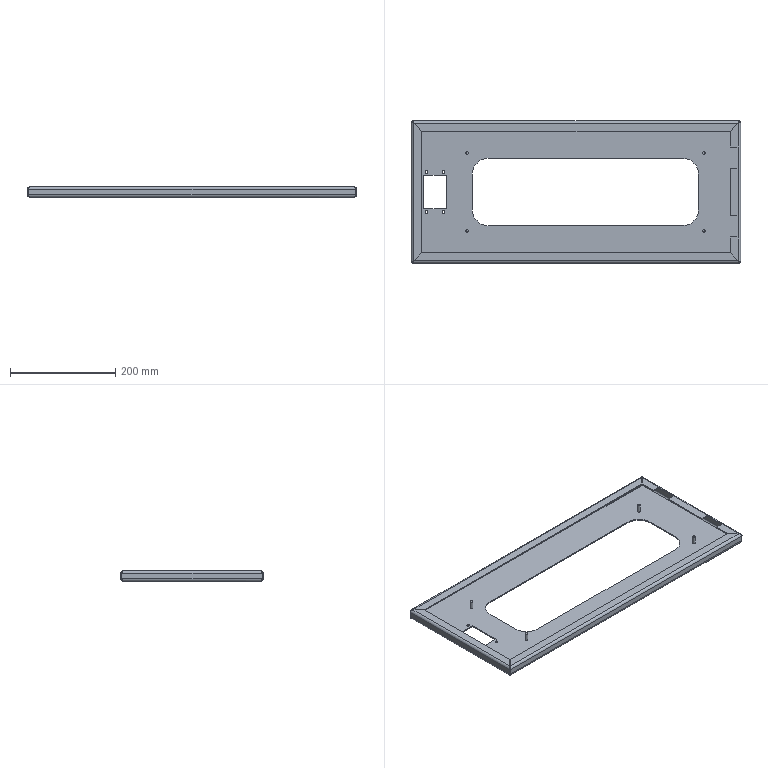Part | SolidWorks | features Cut 3, ICE 2, Fillet 1, FlatPattern 1, MirrorPattern 1, SMBaseFlange 1, SMMiteredFlange 1, SheetMetal 1 | 1 solid | 114 faces | box 626 x 271 x 20 mm | volume 336967 mm3 | plane 62 | cylinder 36 | spline 16 | commonest cylinder face diameters 5 x16 6 x8 10 x8 60 x4